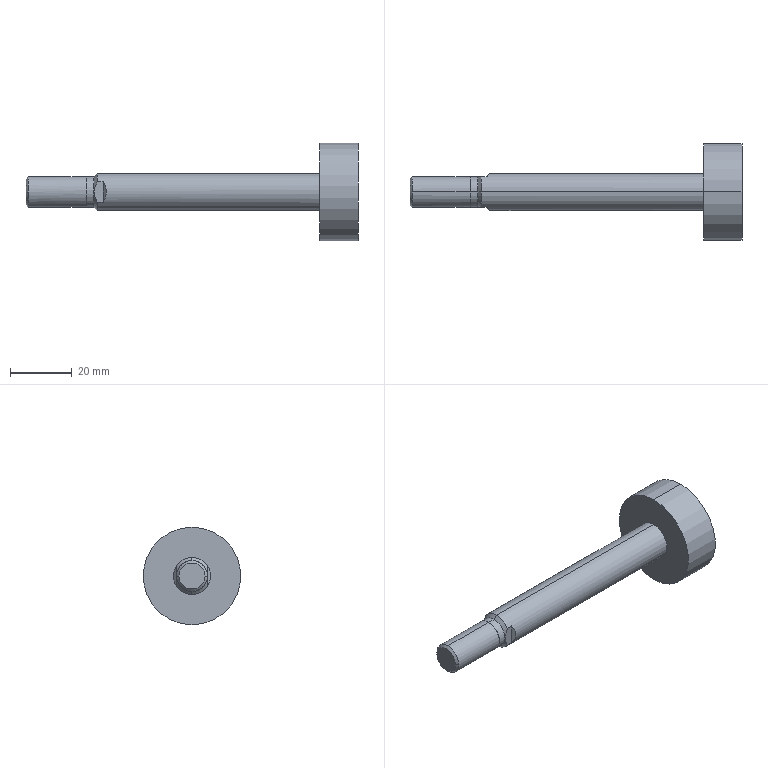Part | STEP file | 11-_MD 32x40-S40 - RodCW11 | 1 solid | 20 faces | box 107.5 x 31.6 x 31.6 mm | volume 19658 mm3 | cylinder 8 | plane 8 | cone 4 | commonest cylinder face diameters 9.8 x2 10 x2 12 x2 31.6 x2
STEP:
#1=CARTESIAN_POINT('',(68.1,0.,6.));
#2=VERTEX_POINT('',#1);
#3=CARTESIAN_POINT('',(68.1,0.,-6.));
#4=VERTEX_POINT('',#3);
#5=CARTESIAN_POINT('',(68.1,0.,0.));
#6=DIRECTION('',(-1.,0.,0.));
#7=DIRECTION('',(0.,0.,1.));
#8=AXIS2_PLACEMENT_3D('',#5,#6,#7);
#9=CIRCLE('',#8,6.);
#10=EDGE_CURVE('',#2,#4,#9,.T.);
#11=ORIENTED_EDGE('',*,*,#10,.T.);
#12=CARTESIAN_POINT('',(-3.9,0.,-6.));
#13=VERTEX_POINT('',#12);
#14=CARTESIAN_POINT('',(80.5,0.,-6.));
#15=DIRECTION('',(-1.,0.,0.));
#16=VECTOR('',#15,1000.);
#17=LINE('',#14,#16);
#18=EDGE_CURVE('',#4,#13,#17,.T.);
#19=ORIENTED_EDGE('',*,*,#18,.T.);
#20=CARTESIAN_POINT('',(-3.9,5.,-3.317));
#21=VERTEX_POINT('',#20);
#22=CARTESIAN_POINT('',(-3.9,0.,0.));
#23=DIRECTION('',(1.,0.,0.));
#24=DIRECTION('',(0.,0.,1.));
#25=AXIS2_PLACEMENT_3D('',#22,#23,#24);
#26=CIRCLE('',#25,6.);
#27=EDGE_CURVE('',#13,#21,#26,.T.);
#28=ORIENTED_EDGE('',*,*,#27,.T.);
#29=CARTESIAN_POINT('',(-2.,5.,-3.317));
#30=VERTEX_POINT('',#29);
#31=CARTESIAN_POINT('',(80.5,5.,-3.317));
#32=DIRECTION('',(1.,0.,0.));
#33=VECTOR('',#32,1000.);
#34=LINE('',#31,#33);
#35=EDGE_CURVE('',#21,#30,#34,.T.);
#36=ORIENTED_EDGE('',*,*,#35,.T.);
#37=CARTESIAN_POINT('',(-2.,5.,3.317));
#38=VERTEX_POINT('',#37);
#39=CARTESIAN_POINT('',(-2.,5.,-3.317));
#40=CARTESIAN_POINT('',(-0.625,6.375,-1.244));
#41=CARTESIAN_POINT('',(-0.625,6.375,1.244));
#42=CARTESIAN_POINT('',(-2.,5.,3.317));
#43=(BOUNDED_CURVE()B_SPLINE_CURVE(3,(#39,#40,#41,#42),.UNSPECIFIED.,.F.,.F.)B_SPLINE_CURVE_WITH_KNOTS((4,4),(2.556,3.727),.UNSPECIFIED.)CURVE()GEOMETRIC_REPRESENTATION_ITEM()RATIONAL_B_SPLINE_CURVE((1.,0.8889,0.8889,1.))REPRESENTATION_ITEM(''));
#44=EDGE_CURVE('',#30,#38,#43,.T.);
#45=ORIENTED_EDGE('',*,*,#44,.T.);
#46=CARTESIAN_POINT('',(-3.9,5.,3.317));
#47=VERTEX_POINT('',#46);
#48=CARTESIAN_POINT('',(80.5,5.,3.317));
#49=DIRECTION('',(-1.,0.,0.));
#50=VECTOR('',#49,1000.);
#51=LINE('',#48,#50);
#52=EDGE_CURVE('',#38,#47,#51,.T.);
#53=ORIENTED_EDGE('',*,*,#52,.T.);
#54=CARTESIAN_POINT('',(-3.9,0.,6.));
#55=VERTEX_POINT('',#54);
#56=CARTESIAN_POINT('',(-3.9,0.,0.));
#57=DIRECTION('',(1.,0.,0.));
#58=DIRECTION('',(0.,0.,1.));
#59=AXIS2_PLACEMENT_3D('',#56,#57,#58);
#60=CIRCLE('',#59,6.);
#61=EDGE_CURVE('',#47,#55,#60,.T.);
#62=ORIENTED_EDGE('',*,*,#61,.T.);
#63=CARTESIAN_POINT('',(80.5,0.,6.));
#64=DIRECTION('',(-1.,0.,0.));
#65=VECTOR('',#64,1000.);
#66=LINE('',#63,#65);
#67=EDGE_CURVE('',#2,#55,#66,.T.);
#68=ORIENTED_EDGE('',*,*,#67,.F.);
#69=EDGE_LOOP('',(#11,#19,#28,#36,#45,#53,#62,#68));
#70=FACE_OUTER_BOUND('',#69,.T.);
#71=CARTESIAN_POINT('',(80.5,0.,0.));
#72=DIRECTION('',(-1.,0.,0.));
#73=DIRECTION('',(0.,0.,1.));
#74=AXIS2_PLACEMENT_3D('',#71,#72,#73);
#75=CYLINDRICAL_SURFACE('',#74,6.);
#76=ADVANCED_FACE('',(#70),#75,.T.);
#77=CARTESIAN_POINT('',(-5.,0.,-4.9));
#78=VERTEX_POINT('',#77);
#79=CARTESIAN_POINT('',(-5.,0.,4.9));
#80=VERTEX_POINT('',#79);
#81=CARTESIAN_POINT('',(-5.,0.,0.));
#82=DIRECTION('',(1.,0.,0.));
#83=DIRECTION('',(0.,0.,-1.));
#84=AXIS2_PLACEMENT_3D('',#81,#82,#83);
#85=CIRCLE('',#84,4.9);
#86=EDGE_CURVE('',#78,#80,#85,.T.);
#87=ORIENTED_EDGE('',*,*,#86,.T.);
#88=CARTESIAN_POINT('',(-3.9,0.,6.));
#89=DIRECTION('',(0.7071,0.,0.7071));
#90=VECTOR('',#89,1000.);
#91=LINE('',#88,#90);
#92=EDGE_CURVE('',#80,#55,#91,.T.);
#93=ORIENTED_EDGE('',*,*,#92,.T.);
#94=ORIENTED_EDGE('',*,*,#61,.F.);
#95=CARTESIAN_POINT('',(-3.9,5.,3.317));
#96=CARTESIAN_POINT('',(-4.183,5.,2.804));
#97=CARTESIAN_POINT('',(-4.431,5.,2.277));
#98=CARTESIAN_POINT('',(-4.701,5.,1.447));
#99=CARTESIAN_POINT('',(-4.775,5.,1.161));
#100=CARTESIAN_POINT('',(-4.874,5.,0.583));
#101=CARTESIAN_POINT('',(-4.9,5.,0.2931));
#102=CARTESIAN_POINT('',(-4.9,5.,-0.2881));
#103=CARTESIAN_POINT('',(-4.874,5.,-0.5813));
#104=CARTESIAN_POINT('',(-4.775,5.,-1.161));
#105=CARTESIAN_POINT('',(-4.703,5.,-1.443));
#106=CARTESIAN_POINT('',(-4.433,5.,-2.272));
#107=CARTESIAN_POINT('',(-4.184,5.,-2.803));
#108=CARTESIAN_POINT('',(-3.9,5.,-3.317));
#109=B_SPLINE_CURVE_WITH_KNOTS('',3,(#95,#96,#97,#98,#99,#100,#101,#102,#103,#104,#105,#106,#107,#108),.UNSPECIFIED.,.F.,.F.,(4,2,2,2,2,2,4),(0.,0.001743,0.002614,0.003485,0.004357,0.005228,0.006971),.UNSPECIFIED.);
#110=EDGE_CURVE('',#47,#21,#109,.T.);
#111=ORIENTED_EDGE('',*,*,#110,.T.);
#112=ORIENTED_EDGE('',*,*,#27,.F.);
#113=CARTESIAN_POINT('',(-3.9,0.,-6.));
#114=DIRECTION('',(0.7071,0.,-0.7071));
#115=VECTOR('',#114,1000.);
#116=LINE('',#113,#115);
#117=EDGE_CURVE('',#78,#13,#116,.T.);
#118=ORIENTED_EDGE('',*,*,#117,.F.);
#119=EDGE_LOOP('',(#87,#93,#94,#111,#112,#118));
#120=FACE_OUTER_BOUND('',#119,.T.);
#121=CARTESIAN_POINT('',(-3.9,0.,0.));
#122=DIRECTION('',(1.,0.,0.));
#123=DIRECTION('',(0.,0.,-1.));
#124=AXIS2_PLACEMENT_3D('',#121,#122,#123);
#125=CONICAL_SURFACE('',#124,6.,0.7854);
#126=ADVANCED_FACE('',(#120),#125,.T.);
#127=ORIENTED_EDGE('',*,*,#86,.F.);
#128=CARTESIAN_POINT('',(-7.5,0.,-4.9));
#129=VERTEX_POINT('',#128);
#130=CARTESIAN_POINT('',(80.5,0.,-4.9));
#131=DIRECTION('',(-1.,0.,0.));
#132=VECTOR('',#131,1000.);
#133=LINE('',#130,#132);
#134=EDGE_CURVE('',#78,#129,#133,.T.);
#135=ORIENTED_EDGE('',*,*,#134,.T.);
#136=CARTESIAN_POINT('',(-7.5,0.,4.9));
#137=VERTEX_POINT('',#136);
#138=CARTESIAN_POINT('',(-7.5,0.,0.));
#139=DIRECTION('',(1.,0.,0.));
#140=DIRECTION('',(0.,0.,1.));
#141=AXIS2_PLACEMENT_3D('',#138,#139,#140);
#142=CIRCLE('',#141,4.9);
#143=EDGE_CURVE('',#129,#137,#142,.T.);
#144=ORIENTED_EDGE('',*,*,#143,.T.);
#145=CARTESIAN_POINT('',(80.5,0.,4.9));
#146=DIRECTION('',(-1.,0.,0.));
#147=VECTOR('',#146,1000.);
#148=LINE('',#145,#147);
#149=EDGE_CURVE('',#80,#137,#148,.T.);
#150=ORIENTED_EDGE('',*,*,#149,.F.);
#151=EDGE_LOOP('',(#127,#135,#144,#150));
#152=FACE_OUTER_BOUND('',#151,.T.);
#153=CARTESIAN_POINT('',(80.5,0.,0.));
#154=DIRECTION('',(-1.,0.,0.));
#155=DIRECTION('',(0.,0.,1.));
#156=AXIS2_PLACEMENT_3D('',#153,#154,#155);
#157=CYLINDRICAL_SURFACE('',#156,4.9);
#158=ADVANCED_FACE('',(#152),#157,.T.);
#159=CARTESIAN_POINT('',(80.5,0.,15.8));
#160=VERTEX_POINT('',#159);
#161=CARTESIAN_POINT('',(80.5,0.,-15.8));
#162=VERTEX_POINT('',#161);
#163=CARTESIAN_POINT('',(80.5,0.,0.));
#164=DIRECTION('',(-1.,0.,0.));
#165=DIRECTION('',(0.,0.,1.));
#166=AXIS2_PLACEMENT_3D('',#163,#164,#165);
#167=CIRCLE('',#166,15.8);
#168=EDGE_CURVE('',#160,#162,#167,.T.);
#169=ORIENTED_EDGE('',*,*,#168,.T.);
#170=CARTESIAN_POINT('',(68.1,0.,-15.8));
#171=VERTEX_POINT('',#170);
#172=CARTESIAN_POINT('',(80.5,0.,-15.8));
#173=DIRECTION('',(-1.,0.,0.));
#174=VECTOR('',#173,1000.);
#175=LINE('',#172,#174);
#176=EDGE_CURVE('',#162,#171,#175,.T.);
#177=ORIENTED_EDGE('',*,*,#176,.T.);
#178=CARTESIAN_POINT('',(68.1,0.,15.8));
#179=VERTEX_POINT('',#178);
#180=CARTESIAN_POINT('',(68.1,0.,0.));
#181=DIRECTION('',(1.,0.,0.));
#182=DIRECTION('',(0.,0.,1.));
#183=AXIS2_PLACEMENT_3D('',#180,#181,#182);
#184=CIRCLE('',#183,15.8);
#185=EDGE_CURVE('',#171,#179,#184,.T.);
#186=ORIENTED_EDGE('',*,*,#185,.T.);
#187=CARTESIAN_POINT('',(80.5,0.,15.8));
#188=DIRECTION('',(-1.,0.,0.));
#189=VECTOR('',#188,1000.);
#190=LINE('',#187,#189);
#191=EDGE_CURVE('',#160,#179,#190,.T.);
#192=ORIENTED_EDGE('',*,*,#191,.F.);
#193=EDGE_LOOP('',(#169,#177,#186,#192));
#194=FACE_OUTER_BOUND('',#193,.T.);
#195=CARTESIAN_POINT('',(80.5,0.,0.));
#196=DIRECTION('',(-1.,0.,0.));
#197=DIRECTION('',(0.,0.,1.));
#198=AXIS2_PLACEMENT_3D('',#195,#196,#197);
#199=CYLINDRICAL_SURFACE('',#198,15.8);
#200=ADVANCED_FACE('',(#194),#199,.T.);
#201=CARTESIAN_POINT('',(-7.5,0.,5.));
#202=VERTEX_POINT('',#201);
#203=CARTESIAN_POINT('',(-7.5,0.,-5.));
#204=VERTEX_POINT('',#203);
#205=CARTESIAN_POINT('',(-7.5,0.,0.));
#206=DIRECTION('',(-1.,0.,0.));
#207=DIRECTION('',(0.,0.,1.));
#208=AXIS2_PLACEMENT_3D('',#205,#206,#207);
#209=CIRCLE('',#208,5.);
#210=EDGE_CURVE('',#202,#204,#209,.T.);
#211=ORIENTED_EDGE('',*,*,#210,.T.);
#212=CARTESIAN_POINT('',(-26.233,0.,-5.));
#213=VERTEX_POINT('',#212);
#214=CARTESIAN_POINT('',(80.5,0.,-5.));
#215=DIRECTION('',(-1.,0.,0.));
#216=VECTOR('',#215,1000.);
#217=LINE('',#214,#216);
#218=EDGE_CURVE('',#204,#213,#217,.T.);
#219=ORIENTED_EDGE('',*,*,#218,.T.);
#220=CARTESIAN_POINT('',(-26.233,5.,0.));
#221=VERTEX_POINT('',#220);
#222=CARTESIAN_POINT('',(-26.233,0.,0.));
#223=DIRECTION('',(1.,0.,0.));
#224=DIRECTION('',(0.,0.,1.));
#225=AXIS2_PLACEMENT_3D('',#222,#223,#224);
#226=CIRCLE('',#225,5.);
#227=EDGE_CURVE('',#213,#221,#226,.T.);
#228=ORIENTED_EDGE('',*,*,#227,.T.);
#229=CARTESIAN_POINT('',(-26.233,0.,5.));
#230=VERTEX_POINT('',#229);
#231=CARTESIAN_POINT('',(-26.233,0.,0.));
#232=DIRECTION('',(1.,0.,0.));
#233=DIRECTION('',(0.,0.,1.));
#234=AXIS2_PLACEMENT_3D('',#231,#232,#233);
#235=CIRCLE('',#234,5.);
#236=EDGE_CURVE('',#221,#230,#235,.T.);
#237=ORIENTED_EDGE('',*,*,#236,.T.);
#238=CARTESIAN_POINT('',(80.5,0.,5.));
#239=DIRECTION('',(-1.,0.,0.));
#240=VECTOR('',#239,1000.);
#241=LINE('',#238,#240);
#242=EDGE_CURVE('',#202,#230,#241,.T.);
#243=ORIENTED_EDGE('',*,*,#242,.F.);
#244=EDGE_LOOP('',(#211,#219,#228,#237,#243));
#245=FACE_OUTER_BOUND('',#244,.T.);
#246=CARTESIAN_POINT('',(80.5,0.,0.));
#247=DIRECTION('',(-1.,0.,0.));
#248=DIRECTION('',(0.,0.,1.));
#249=AXIS2_PLACEMENT_3D('',#246,#247,#248);
#250=CYLINDRICAL_SURFACE('',#249,5.);
#251=ADVANCED_FACE('',(#245),#250,.T.);
#252=CARTESIAN_POINT('',(-27.,4.233,0.));
#253=VERTEX_POINT('',#252);
#254=CARTESIAN_POINT('',(-27.,-4.233,0.));
#255=VERTEX_POINT('',#254);
#256=CARTESIAN_POINT('',(-27.,0.,0.));
#257=DIRECTION('',(1.,0.,0.));
#258=DIRECTION('',(0.,1.,0.));
#259=AXIS2_PLACEMENT_3D('',#256,#257,#258);
#260=CIRCLE('',#259,4.233);
#261=EDGE_CURVE('',#253,#255,#260,.T.);
#262=ORIENTED_EDGE('',*,*,#261,.T.);
#263=CARTESIAN_POINT('',(-26.233,-5.,0.));
#264=VERTEX_POINT('',#263);
#265=CARTESIAN_POINT('',(-26.233,-5.,0.));
#266=DIRECTION('',(0.7071,-0.7071,0.));
#267=VECTOR('',#266,1000.);
#268=LINE('',#265,#267);
#269=EDGE_CURVE('',#255,#264,#268,.T.);
#270=ORIENTED_EDGE('',*,*,#269,.T.);
#271=CARTESIAN_POINT('',(-26.233,0.,0.));
#272=DIRECTION('',(1.,0.,0.));
#273=DIRECTION('',(0.,0.,1.));
#274=AXIS2_PLACEMENT_3D('',#271,#272,#273);
#275=CIRCLE('',#274,5.);
#276=EDGE_CURVE('',#230,#264,#275,.T.);
#277=ORIENTED_EDGE('',*,*,#276,.F.);
#278=ORIENTED_EDGE('',*,*,#236,.F.);
#279=CARTESIAN_POINT('',(-26.233,5.,0.));
#280=DIRECTION('',(0.7071,0.7071,0.));
#281=VECTOR('',#280,1000.);
#282=LINE('',#279,#281);
#283=EDGE_CURVE('',#253,#221,#282,.T.);
#284=ORIENTED_EDGE('',*,*,#283,.F.);
#285=EDGE_LOOP('',(#262,#270,#277,#278,#284));
#286=FACE_OUTER_BOUND('',#285,.T.);
#287=CARTESIAN_POINT('',(-26.233,0.,0.));
#288=DIRECTION('',(1.,0.,0.));
#289=DIRECTION('',(0.,1.,0.));
#290=AXIS2_PLACEMENT_3D('',#287,#288,#289);
#291=CONICAL_SURFACE('',#290,5.,0.7854);
#292=ADVANCED_FACE('',(#286),#291,.T.);
#293=ORIENTED_EDGE('',*,*,#18,.F.);
#294=CARTESIAN_POINT('',(68.1,0.,0.));
#295=DIRECTION('',(-1.,0.,0.));
#296=DIRECTION('',(0.,0.,1.));
#297=AXIS2_PLACEMENT_3D('',#294,#295,#296);
#298=CIRCLE('',#297,6.);
#299=EDGE_CURVE('',#4,#2,#298,.T.);
#300=ORIENTED_EDGE('',*,*,#299,.T.);
#301=ORIENTED_EDGE('',*,*,#67,.T.);
#302=CARTESIAN_POINT('',(-3.9,-5.,3.317));
#303=VERTEX_POINT('',#302);
#304=CARTESIAN_POINT('',(-3.9,0.,0.));
#305=DIRECTION('',(1.,0.,0.));
#306=DIRECTION('',(0.,0.,1.));
#307=AXIS2_PLACEMENT_3D('',#304,#305,#306);
#308=CIRCLE('',#307,6.);
#309=EDGE_CURVE('',#55,#303,#308,.T.);
#310=ORIENTED_EDGE('',*,*,#309,.T.);
#311=CARTESIAN_POINT('',(-2.,-5.,3.317));
#312=VERTEX_POINT('',#311);
#313=CARTESIAN_POINT('',(80.5,-5.,3.317));
#314=DIRECTION('',(1.,0.,0.));
#315=VECTOR('',#314,1000.);
#316=LINE('',#313,#315);
#317=EDGE_CURVE('',#303,#312,#316,.T.);
#318=ORIENTED_EDGE('',*,*,#317,.T.);
#319=CARTESIAN_POINT('',(-2.,-5.,-3.317));
#320=VERTEX_POINT('',#319);
#321=CARTESIAN_POINT('',(-2.,-5.,3.317));
#322=CARTESIAN_POINT('',(-0.625,-6.375,1.244));
#323=CARTESIAN_POINT('',(-0.625,-6.375,-1.244));
#324=CARTESIAN_POINT('',(-2.,-5.,-3.317));
#325=(BOUNDED_CURVE()B_SPLINE_CURVE(3,(#321,#322,#323,#324),.UNSPECIFIED.,.F.,.F.)B_SPLINE_CURVE_WITH_KNOTS((4,4),(2.556,3.727),.UNSPECIFIED.)CURVE()GEOMETRIC_REPRESENTATION_ITEM()RATIONAL_B_SPLINE_CURVE((1.,0.8889,0.8889,1.))REPRESENTATION_ITEM(''));
#326=EDGE_CURVE('',#312,#320,#325,.T.);
#327=ORIENTED_EDGE('',*,*,#326,.T.);
#328=CARTESIAN_POINT('',(-3.9,-5.,-3.317));
#329=VERTEX_POINT('',#328);
#330=CARTESIAN_POINT('',(80.5,-5.,-3.317));
#331=DIRECTION('',(-1.,0.,0.));
#332=VECTOR('',#331,1000.);
#333=LINE('',#330,#332);
#334=EDGE_CURVE('',#320,#329,#333,.T.);
#335=ORIENTED_EDGE('',*,*,#334,.T.);
#336=CARTESIAN_POINT('',(-3.9,0.,0.));
#337=DIRECTION('',(1.,0.,0.));
#338=DIRECTION('',(0.,0.,1.));
#339=AXIS2_PLACEMENT_3D('',#336,#337,#338);
#340=CIRCLE('',#339,6.);
#341=EDGE_CURVE('',#329,#13,#340,.T.);
#342=ORIENTED_EDGE('',*,*,#341,.T.);
#343=EDGE_LOOP('',(#293,#300,#301,#310,#318,#327,#335,#342));
#344=FACE_OUTER_BOUND('',#343,.T.);
#345=CARTESIAN_POINT('',(80.5,0.,0.));
#346=DIRECTION('',(-1.,0.,0.));
#347=DIRECTION('',(0.,0.,1.));
#348=AXIS2_PLACEMENT_3D('',#345,#346,#347);
#349=CYLINDRICAL_SURFACE('',#348,6.);
#350=ADVANCED_FACE('',(#344),#349,.T.);
#351=ORIENTED_EDGE('',*,*,#317,.F.);
#352=CARTESIAN_POINT('',(-3.9,-5.,3.317));
#353=CARTESIAN_POINT('',(-4.183,-5.,2.804));
#354=CARTESIAN_POINT('',(-4.431,-5.,2.277));
#355=CARTESIAN_POINT('',(-4.701,-5.,1.447));
#356=CARTESIAN_POINT('',(-4.775,-5.,1.161));
#357=CARTESIAN_POINT('',(-4.874,-5.,0.583));
#358=CARTESIAN_POINT('',(-4.9,-5.,0.2931));
#359=CARTESIAN_POINT('',(-4.9,-5.,-0.2881));
#360=CARTESIAN_POINT('',(-4.874,-5.,-0.5813));
#361=CARTESIAN_POINT('',(-4.775,-5.,-1.161));
#362=CARTESIAN_POINT('',(-4.703,-5.,-1.443));
#363=CARTESIAN_POINT('',(-4.433,-5.,-2.272));
#364=CARTESIAN_POINT('',(-4.184,-5.,-2.803));
#365=CARTESIAN_POINT('',(-3.9,-5.,-3.317));
#366=B_SPLINE_CURVE_WITH_KNOTS('',3,(#352,#353,#354,#355,#356,#357,#358,#359,#360,#361,#362,#363,#364,#365),.UNSPECIFIED.,.F.,.F.,(4,2,2,2,2,2,4),(0.,0.001743,0.002614,0.003485,0.004357,0.005228,0.006971),.UNSPECIFIED.);
#367=EDGE_CURVE('',#303,#329,#366,.T.);
#368=ORIENTED_EDGE('',*,*,#367,.T.);
#369=ORIENTED_EDGE('',*,*,#334,.F.);
#370=CARTESIAN_POINT('',(-2.,-5.,12.));
#371=DIRECTION('',(0.,0.,1.));
#372=VECTOR('',#371,1000.);
#373=LINE('',#370,#372);
#374=EDGE_CURVE('',#320,#312,#373,.T.);
#375=ORIENTED_EDGE('',*,*,#374,.T.);
#376=EDGE_LOOP('',(#351,#368,#369,#375));
#377=FACE_OUTER_BOUND('',#376,.T.);
#378=CARTESIAN_POINT('',(-2.,-5.,12.));
#379=DIRECTION('',(0.,-1.,0.));
#380=DIRECTION('',(0.,0.,-1.));
#381=AXIS2_PLACEMENT_3D('',#378,#379,#380);
#382=PLANE('',#381);
#383=ADVANCED_FACE('',(#377),#382,.T.);
#384=ORIENTED_EDGE('',*,*,#92,.F.);
#385=CARTESIAN_POINT('',(-5.,0.,0.));
#386=DIRECTION('',(1.,0.,0.));
#387=DIRECTION('',(0.,0.,-1.));
#388=AXIS2_PLACEMENT_3D('',#385,#386,#387);
#389=CIRCLE('',#388,4.9);
#390=EDGE_CURVE('',#80,#78,#389,.T.);
#391=ORIENTED_EDGE('',*,*,#390,.T.);
#392=ORIENTED_EDGE('',*,*,#117,.T.);
#393=ORIENTED_EDGE('',*,*,#341,.F.);
#394=ORIENTED_EDGE('',*,*,#367,.F.);
#395=ORIENTED_EDGE('',*,*,#309,.F.);
#396=EDGE_LOOP('',(#384,#391,#392,#393,#394,#395));
#397=FACE_OUTER_BOUND('',#396,.T.);
#398=CARTESIAN_POINT('',(-3.9,0.,0.));
#399=DIRECTION('',(1.,0.,0.));
#400=DIRECTION('',(0.,0.,-1.));
#401=AXIS2_PLACEMENT_3D('',#398,#399,#400);
#402=CONICAL_SURFACE('',#401,6.,0.7854);
#403=ADVANCED_FACE('',(#397),#402,.T.);
#404=ORIENTED_EDGE('',*,*,#35,.F.);
#405=ORIENTED_EDGE('',*,*,#110,.F.);
#406=ORIENTED_EDGE('',*,*,#52,.F.);
#407=CARTESIAN_POINT('',(-2.,5.,12.));
#408=DIRECTION('',(0.,0.,-1.));
#409=VECTOR('',#408,1000.);
#410=LINE('',#407,#409);
#411=EDGE_CURVE('',#38,#30,#410,.T.);
#412=ORIENTED_EDGE('',*,*,#411,.T.);
#413=EDGE_LOOP('',(#404,#405,#406,#412));
#414=FACE_OUTER_BOUND('',#413,.T.);
#415=CARTESIAN_POINT('',(-31.,5.,12.));
#416=DIRECTION('',(0.,1.,0.));
#417=DIRECTION('',(0.,0.,1.));
#418=AXIS2_PLACEMENT_3D('',#415,#416,#417);
#419=PLANE('',#418);
#420=ADVANCED_FACE('',(#414),#419,.T.);
#421=ORIENTED_EDGE('',*,*,#44,.F.);
#422=ORIENTED_EDGE('',*,*,#411,.F.);
#423=EDGE_LOOP('',(#421,#422));
#424=FACE_OUTER_BOUND('',#423,.T.);
#425=CARTESIAN_POINT('',(-2.,5.,12.));
#426=DIRECTION('',(-0.7071,0.7071,0.));
#427=DIRECTION('',(-0.7071,-0.7071,0.));
#428=AXIS2_PLACEMENT_3D('',#425,#426,#427);
#429=PLANE('',#428);
#430=ADVANCED_FACE('',(#424),#429,.T.);
#431=ORIENTED_EDGE('',*,*,#326,.F.);
#432=ORIENTED_EDGE('',*,*,#374,.F.);
#433=EDGE_LOOP('',(#431,#432));
#434=FACE_OUTER_BOUND('',#433,.T.);
#435=CARTESIAN_POINT('',(-1.,-6.,12.));
#436=DIRECTION('',(-0.7071,-0.7071,0.));
#437=DIRECTION('',(0.7071,-0.7071,0.));
#438=AXIS2_PLACEMENT_3D('',#435,#436,#437);
#439=PLANE('',#438);
#440=ADVANCED_FACE('',(#434),#439,.T.);
#441=ORIENTED_EDGE('',*,*,#10,.F.);
#442=ORIENTED_EDGE('',*,*,#299,.F.);
#443=EDGE_LOOP('',(#441,#442));
#444=FACE_BOUND('',#443,.T.);
#445=CARTESIAN_POINT('',(68.1,0.,0.));
#446=DIRECTION('',(1.,0.,0.));
#447=DIRECTION('',(0.,0.,1.));
#448=AXIS2_PLACEMENT_3D('',#445,#446,#447);
#449=CIRCLE('',#448,15.8);
#450=EDGE_CURVE('',#179,#171,#449,.T.);
#451=ORIENTED_EDGE('',*,*,#450,.F.);
#452=ORIENTED_EDGE('',*,*,#185,.F.);
#453=EDGE_LOOP('',(#451,#452));
#454=FACE_OUTER_BOUND('',#453,.T.);
#455=CARTESIAN_POINT('',(68.1,6.,0.));
#456=DIRECTION('',(1.,0.,0.));
#457=DIRECTION('',(0.,0.,-1.));
#458=AXIS2_PLACEMENT_3D('',#455,#456,#457);
#459=PLANE('',#458);
#460=ADVANCED_FACE('',(#444,#454),#459,.F.);
#461=ORIENTED_EDGE('',*,*,#134,.F.);
#462=ORIENTED_EDGE('',*,*,#390,.F.);
#463=ORIENTED_EDGE('',*,*,#149,.T.);
#464=CARTESIAN_POINT('',(-7.5,0.,0.));
#465=DIRECTION('',(1.,0.,0.));
#466=DIRECTION('',(0.,0.,1.));
#467=AXIS2_PLACEMENT_3D('',#464,#465,#466);
#468=CIRCLE('',#467,4.9);
#469=EDGE_CURVE('',#137,#129,#468,.T.);
#470=ORIENTED_EDGE('',*,*,#469,.T.);
#471=EDGE_LOOP('',(#461,#462,#463,#470));
#472=FACE_OUTER_BOUND('',#471,.T.);
#473=CARTESIAN_POINT('',(80.5,0.,0.));
#474=DIRECTION('',(-1.,0.,0.));
#475=DIRECTION('',(0.,0.,1.));
#476=AXIS2_PLACEMENT_3D('',#473,#474,#475);
#477=CYLINDRICAL_SURFACE('',#476,4.9);
#478=ADVANCED_FACE('',(#472),#477,.T.);
#479=ORIENTED_EDGE('',*,*,#176,.F.);
#480=CARTESIAN_POINT('',(80.5,0.,0.));
#481=DIRECTION('',(-1.,0.,0.));
#482=DIRECTION('',(0.,0.,1.));
#483=AXIS2_PLACEMENT_3D('',#480,#481,#482);
#484=CIRCLE('',#483,15.8);
#485=EDGE_CURVE('',#162,#160,#484,.T.);
#486=ORIENTED_EDGE('',*,*,#485,.T.);
#487=ORIENTED_EDGE('',*,*,#191,.T.);
#488=ORIENTED_EDGE('',*,*,#450,.T.);
#489=EDGE_LOOP('',(#479,#486,#487,#488));
#490=FACE_OUTER_BOUND('',#489,.T.);
#491=CARTESIAN_POINT('',(80.5,0.,0.));
#492=DIRECTION('',(-1.,0.,0.));
#493=DIRECTION('',(0.,0.,1.));
#494=AXIS2_PLACEMENT_3D('',#491,#492,#493);
#495=CYLINDRICAL_SURFACE('',#494,15.8);
#496=ADVANCED_FACE('',(#490),#495,.T.);
#497=ORIENTED_EDGE('',*,*,#210,.F.);
#498=CARTESIAN_POINT('',(-7.5,0.,0.));
#499=DIRECTION('',(-1.,0.,0.));
#500=DIRECTION('',(0.,0.,1.));
#501=AXIS2_PLACEMENT_3D('',#498,#499,#500);
#502=CIRCLE('',#501,5.);
#503=EDGE_CURVE('',#204,#202,#502,.T.);
#504=ORIENTED_EDGE('',*,*,#503,.F.);
#505=EDGE_LOOP('',(#497,#504));
#506=FACE_OUTER_BOUND('',#505,.T.);
#507=ORIENTED_EDGE('',*,*,#469,.F.);
#508=ORIENTED_EDGE('',*,*,#143,.F.);
#509=EDGE_LOOP('',(#507,#508));
#510=FACE_BOUND('',#509,.T.);
#511=CARTESIAN_POINT('',(-7.5,5.,0.));
#512=DIRECTION('',(-1.,0.,0.));
#513=DIRECTION('',(0.,0.,1.));
#514=AXIS2_PLACEMENT_3D('',#511,#512,#513);
#515=PLANE('',#514);
#516=ADVANCED_FACE('',(#506,#510),#515,.F.);
#517=ORIENTED_EDGE('',*,*,#168,.F.);
#518=ORIENTED_EDGE('',*,*,#485,.F.);
#519=EDGE_LOOP('',(#517,#518));
#520=FACE_OUTER_BOUND('',#519,.T.);
#521=CARTESIAN_POINT('',(80.5,15.8,0.));
#522=DIRECTION('',(-1.,0.,0.));
#523=DIRECTION('',(0.,0.,1.));
#524=AXIS2_PLACEMENT_3D('',#521,#522,#523);
#525=PLANE('',#524);
#526=ADVANCED_FACE('',(#520),#525,.F.);
#527=ORIENTED_EDGE('',*,*,#218,.F.);
#528=ORIENTED_EDGE('',*,*,#503,.T.);
#529=ORIENTED_EDGE('',*,*,#242,.T.);
#530=ORIENTED_EDGE('',*,*,#276,.T.);
#531=CARTESIAN_POINT('',(-26.233,0.,0.));
#532=DIRECTION('',(1.,0.,0.));
#533=DIRECTION('',(0.,0.,1.));
#534=AXIS2_PLACEMENT_3D('',#531,#532,#533);
#535=CIRCLE('',#534,5.);
#536=EDGE_CURVE('',#264,#213,#535,.T.);
#537=ORIENTED_EDGE('',*,*,#536,.T.);
#538=EDGE_LOOP('',(#527,#528,#529,#530,#537));
#539=FACE_OUTER_BOUND('',#538,.T.);
#540=CARTESIAN_POINT('',(80.5,0.,0.));
#541=DIRECTION('',(-1.,0.,0.));
#542=DIRECTION('',(0.,0.,1.));
#543=AXIS2_PLACEMENT_3D('',#540,#541,#542);
#544=CYLINDRICAL_SURFACE('',#543,5.);
#545=ADVANCED_FACE('',(#539),#544,.T.);
#546=ORIENTED_EDGE('',*,*,#269,.F.);
#547=CARTESIAN_POINT('',(-27.,0.,0.));
#548=DIRECTION('',(1.,0.,0.));
#549=DIRECTION('',(0.,1.,0.));
#550=AXIS2_PLACEMENT_3D('',#547,#548,#549);
#551=CIRCLE('',#550,4.233);
#552=EDGE_CURVE('',#255,#253,#551,.T.);
#553=ORIENTED_EDGE('',*,*,#552,.T.);
#554=ORIENTED_EDGE('',*,*,#283,.T.);
#555=ORIENTED_EDGE('',*,*,#227,.F.);
#556=ORIENTED_EDGE('',*,*,#536,.F.);
#557=EDGE_LOOP('',(#546,#553,#554,#555,#556));
#558=FACE_OUTER_BOUND('',#557,.T.);
#559=CARTESIAN_POINT('',(-26.233,0.,0.));
#560=DIRECTION('',(1.,0.,0.));
#561=DIRECTION('',(0.,1.,0.));
#562=AXIS2_PLACEMENT_3D('',#559,#560,#561);
#563=CONICAL_SURFACE('',#562,5.,0.7854);
#564=ADVANCED_FACE('',(#558),#563,.T.);
#565=ORIENTED_EDGE('',*,*,#261,.F.);
#566=ORIENTED_EDGE('',*,*,#552,.F.);
#567=EDGE_LOOP('',(#565,#566));
#568=FACE_OUTER_BOUND('',#567,.T.);
#569=CARTESIAN_POINT('',(-27.,0.,0.));
#570=DIRECTION('',(1.,0.,0.));
#571=DIRECTION('',(0.,0.,-1.));
#572=AXIS2_PLACEMENT_3D('',#569,#570,#571);
#573=PLANE('',#572);
#574=ADVANCED_FACE('',(#568),#573,.F.);
#575=CLOSED_SHELL('',(#76,#126,#158,#200,#251,#292,#350,#383,#403,#420,#430,#440,#460,#478,#496,#516,#526,#545,#564,#574));
#576=MANIFOLD_SOLID_BREP('',#575);
#577=CARTESIAN_POINT('',(0.,0.,0.));
#578=DIRECTION('',(0.,0.,1.));
#579=DIRECTION('',(1.,0.,0.));
#580=AXIS2_PLACEMENT_3D('',#577,#578,#579);
#581=(LENGTH_UNIT()NAMED_UNIT(*)SI_UNIT(.MILLI.,.METRE.));
#582=UNCERTAINTY_MEASURE_WITH_UNIT(LENGTH_MEASURE(0.00001),#581,'','');
#583=(NAMED_UNIT(*)PLANE_ANGLE_UNIT()SI_UNIT($,.RADIAN.));
#584=(NAMED_UNIT(*)SI_UNIT($,.STERADIAN.)SOLID_ANGLE_UNIT());
#585=(GEOMETRIC_REPRESENTATION_CONTEXT(3)GLOBAL_UNCERTAINTY_ASSIGNED_CONTEXT((#582))GLOBAL_UNIT_ASSIGNED_CONTEXT((#581,#583,#584))REPRESENTATION_CONTEXT('',''));
#586=ADVANCED_BREP_SHAPE_REPRESENTATION('',(#576,#580),#585);